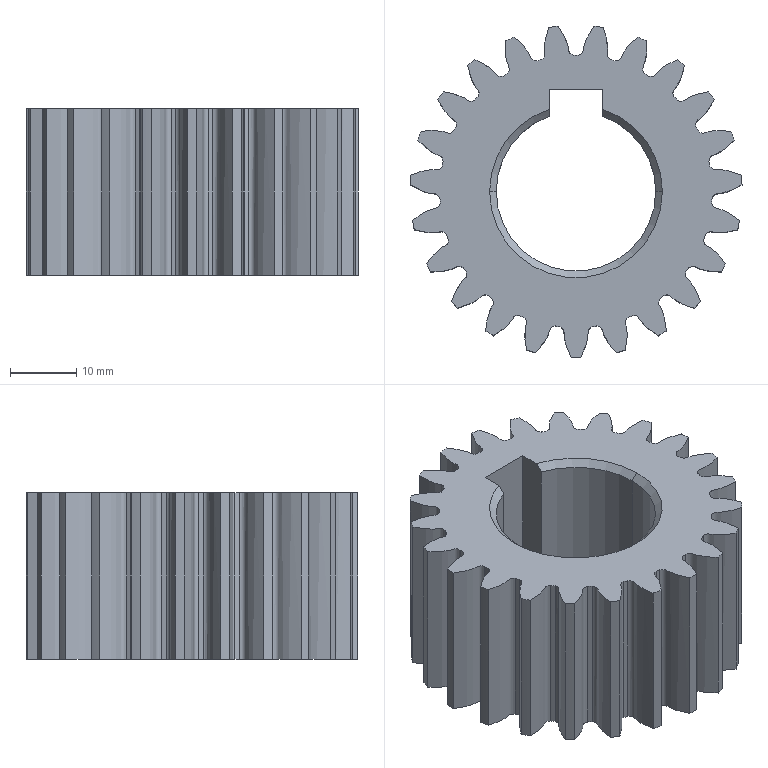Part | SolidWorks | features ICE 3, Chamfer 1, CirPattern 1, Extrusion 1, RefAxis 1 | 1 solid | 106 faces | box 49.96 x 49.854 x 25 mm | volume 28765 mm3 | cylinder 49 | spline 46 | cone 6 | plane 5 | commonest cylinder face diameters 41 x23 50 x23 24 x3